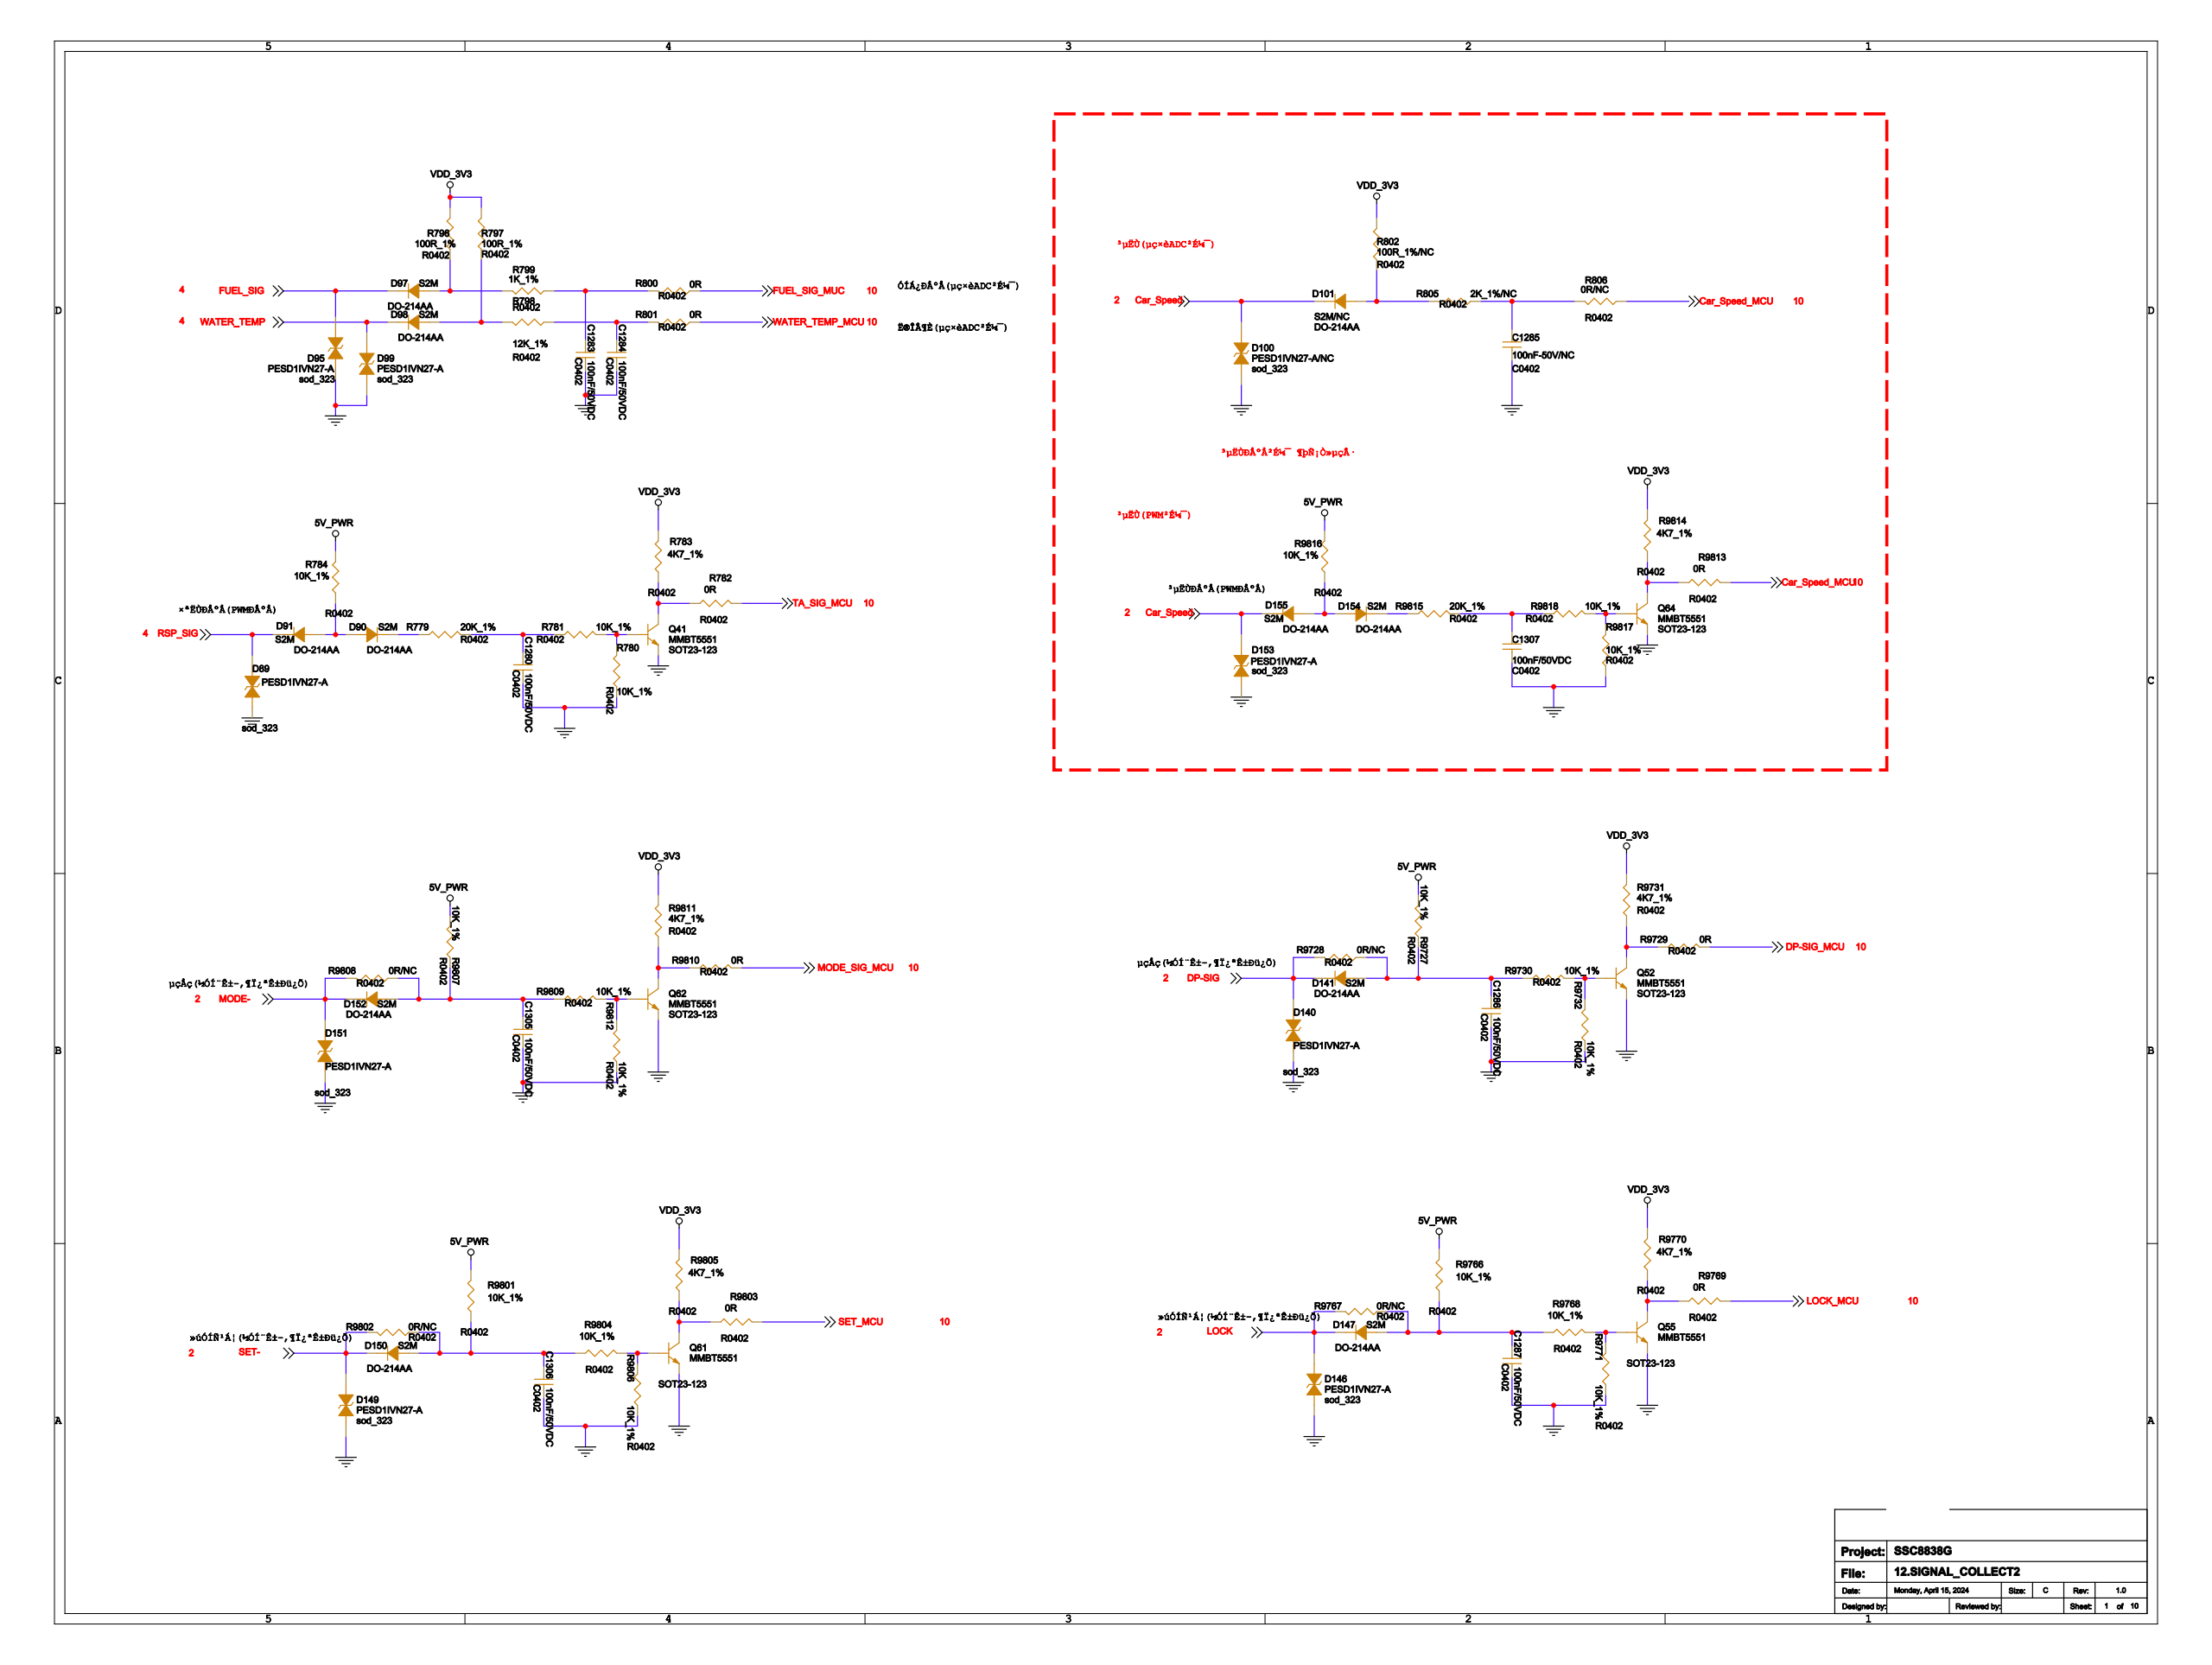Circuit board | Cadence Allegro | 958 parts | 601 nets | one sheet of the schematic
Parts on this sheet (reference | value | footprint):
C1280 | 100nF/50VDC | C0402
C1283 | 100nF/50VDC | C0402
C1284 | 100nF/50VDC | C0402
C1285 | 100nF-50V/NC | C0402
C1286 | 100nF/50VDC | C0402
C1287 | 100nF/50VDC | C0402
C1305 | 100nF/50VDC | C0402
C1306 | 100nF/50VDC | C0402
C1307 | 100nF/50VDC | C0402
D89 | PESD1IVN27-A | SOD_323
D90 | S2M | DO-214AA
D91 | S2M | DO-214AA
D95 | PESD1IVN27-A | SOD_323
D97 | S2M | DO-214AA
D98 | S2M | DO-214AA
D99 | PESD1IVN27-A | SOD_323
D100 | PESD1IVN27-A/NC | SOD_323
D101 | S2M/NC | DO-214AA
D140 | PESD1IVN27-A | SOD_323
D141 | S2M | DO-214AA
D146 | PESD1IVN27-A | SOD_323
D147 | S2M | DO-214AA
D149 | PESD1IVN27-A | SOD_323
D150 | S2M | DO-214AA
D151 | PESD1IVN27-A | SOD_323
D152 | S2M | DO-214AA
D153 | PESD1IVN27-A | SOD_323
D154 | S2M | DO-214AA
D155 | S2M | DO-214AA
Q41 | MMBT5551 | SOT23-123
Q52 | MMBT5551 | SOT23-123
Q55 | MMBT5551 | SOT23-123
Q61 | MMBT5551 | SOT23-123
Q62 | MMBT5551 | SOT23-123
Q64 | MMBT5551 | SOT23-123
R779 | 20K_1% | R0402
R780 | 10K_1% | R0402
R781 | 10K_1% | R0402
R782 | 0R | R0402
R783 | 4K7_1% | R0402
R784 | 10K_1% | R0402
R796 | 100R_1% | R0402
R797 | 100R_1% | R0402
R798 | 12K_1% | R0402
R799 | 1K_1% | R0402
R800 | 0R | R0402
R801 | 0R | R0402
R802 | 100R_1%/NC | R0402
R805 | 2K_1%/NC | R0402
R806 | 0R/NC | R0402
R9727 | 10K_1% | R0402
R9728 | 0R/NC | R0402
R9729 | 0R | R0402
R9730 | 10K_1% | R0402
R9731 | 4K7_1% | R0402
R9732 | 10K_1% | R0402
R9766 | 10K_1% | R0402
R9767 | 0R/NC | R0402
R9768 | 10K_1% | R0402
R9769 | 0R | R0402
R9770 | 4K7_1% | R0402
R9771 | 10K_1% | R0402
R9801 | 10K_1% | R0402
R9802 | 0R/NC | R0402
R9803 | 0R | R0402
R9804 | 10K_1% | R0402
R9805 | 4K7_1% | R0402
R9806 | 10K_1% | R0402
R9807 | 10K_1% | R0402
R9808 | 0R/NC | R0402
R9809 | 10K_1% | R0402
R9810 | 0R | R0402
R9811 | 4K7_1% | R0402
R9812 | 10K_1% | R0402
R9813 | 0R | R0402
R9814 | 4K7_1% | R0402
R9815 | 20K_1% | R0402
R9816 | 10K_1% | R0402
R9817 | 10K_1% | R0402
R9818 | 10K_1% | R0402
Nets of these parts (net: part-pin ...):
GND: C1280-2 C1283-2 C1284-2 C1285-2 C1286-2 C1287-2 C1305-2 C1306-2 C1307-2 D89-1 D95-1 D99-1 D100-1 D140-1 D146-1 D149-1 D151-1 D153-1 Q41-2 Q52-2 Q55-2 Q61-2 Q62-2 Q64-2 R780-1 R9732-1 R9771-1 R9806-1 R9812-1 R9817-1
5V_PWR: R784-2 R9727-2 R9766-2 R9801-2 R9807-2 R9816-2
3V3_NORMAL: R783-2 R796-2 R797-2 R802-2 R9731-2 R9770-2 R9805-2 R9811-2 R9814-2
N21197710: C1280-1 R779-2 R781-1
N21199821: C1283-1 R799-1 R800-2
N21199824: C1284-1 R798-1 R801-2
N21377187: C1286-1 D141-1 R9727-1 R9728-1 R9730-1
N21477459: C1287-1 D147-1 R9766-1 R9767-2 R9768-1
N22030712: C1305-1 D152-1 R9807-1 R9808-1 R9809-1
N22030543: C1306-1 D150-1 R9801-1 R9802-2 R9804-1
N22111311: C1307-1 R9815-2 R9818-1
N21200314: C1285-1 R805-1 R806-2
CAR_SPEED: D100-2 D101-2 D153-2 D155-2
N21200228: D101-1 R802-1 R805-2
DP-SIG: D140-2 D141-2 R9728-2
LOCK: D146-2 D147-2 R9767-1
SET-: D149-2 D150-2 R9802-1
MODE-: D151-2 D152-2 R9808-2
RSP_SIG: D89-2 D91-2
FUEL_SIG: D95-2 D97-2
WATER_TEMP: D98-2 D99-2
N22111339: D154-1 D155-1 R9816-1
N22111347: D154-2 R9815-1
N21197816: D90-1 D91-1 R784-1
N21213729: D90-2 R779-1
N21198848: D97-1 R796-1 R799-2
N21199772: D98-1 R797-1 R798-2
N21197722: Q41-1 R780-2 R781-2
N21197770: Q41-3 R782-1 R783-1
N21377306: Q52-1 R9730-2 R9732-2
N21377339: Q52-3 R9729-1 R9731-1
N21477603: Q55-1 R9768-2 R9771-2
N21477607: Q55-3 R9769-1 R9770-1
N22030539: Q61-1 R9804-2 R9806-2
N22030684: Q61-3 R9803-1 R9805-1
N22030700: Q62-1 R9809-2 R9812-2
N22030848: Q62-3 R9810-1 R9811-1
N22111181: Q64-1 R9817-2 R9818-2
N22111329: Q64-3 R9813-1 R9814-1
TA_SIG_MCU: R782-2
FUEL_SIG_MUC: R800-1
WATER_TEMP_MCU: R801-1
DP-SIG_MCU: R9729-2
LOCK_MCU: R9769-2
SET_MCU: R9803-2
MODE_SIG_MCU: R9810-2
CAR_SPEED_MCU: R806-1 R9813-2